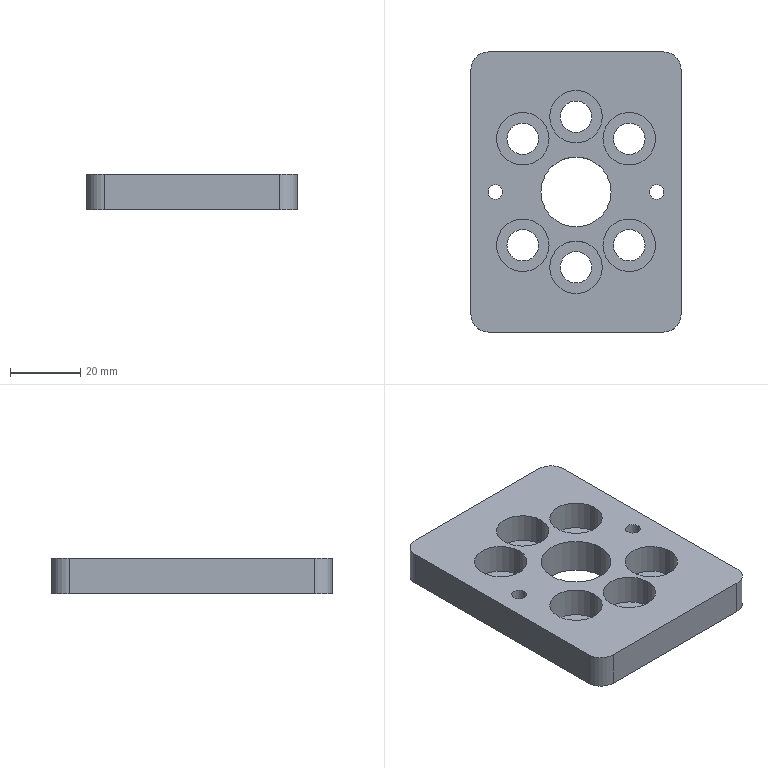Part | SolidWorks | features HoleWzd 2, CirPattern 1, Extrusion 1, Fillet 1 | 1 solid | 46 faces | box 60 x 80 x 10 mm | volume 34714 mm3 | cylinder 34 | plane 12 | commonest cylinder face diameters 9 x12 15 x12 4.2 x4 10 x4 20 x2
STEP:
#1=CARTESIAN_POINT('',(7.703,15.203,1.4));
#2=VERTEX_POINT('',#1);
#3=CARTESIAN_POINT('',(22.703,15.203,1.4));
#4=VERTEX_POINT('',#3);
#5=CARTESIAN_POINT('',(15.203,15.203,1.4));
#6=DIRECTION('',(0.,0.,1.));
#7=DIRECTION('',(1.,0.,0.));
#8=AXIS2_PLACEMENT_3D('',#5,#6,#7);
#9=CIRCLE('',#8,7.5);
#10=EDGE_CURVE('',#2,#4,#9,.T.);
#11=ORIENTED_EDGE('',*,*,#10,.F.);
#12=CARTESIAN_POINT('',(7.703,15.203,10.));
#13=VERTEX_POINT('',#12);
#14=CARTESIAN_POINT('',(7.703,15.203,10.));
#15=DIRECTION('',(0.,0.,1.));
#16=VECTOR('',#15,1000.);
#17=LINE('',#14,#16);
#18=EDGE_CURVE('',#2,#13,#17,.T.);
#19=ORIENTED_EDGE('',*,*,#18,.T.);
#20=CARTESIAN_POINT('',(22.703,15.203,10.));
#21=VERTEX_POINT('',#20);
#22=CARTESIAN_POINT('',(15.203,15.203,10.));
#23=DIRECTION('',(0.,0.,1.));
#24=DIRECTION('',(1.,0.,0.));
#25=AXIS2_PLACEMENT_3D('',#22,#23,#24);
#26=CIRCLE('',#25,7.5);
#27=EDGE_CURVE('',#13,#21,#26,.T.);
#28=ORIENTED_EDGE('',*,*,#27,.T.);
#29=CARTESIAN_POINT('',(22.703,15.203,10.));
#30=DIRECTION('',(0.,0.,1.));
#31=VECTOR('',#30,1000.);
#32=LINE('',#29,#31);
#33=EDGE_CURVE('',#4,#21,#32,.T.);
#34=ORIENTED_EDGE('',*,*,#33,.F.);
#35=EDGE_LOOP('',(#11,#19,#28,#34));
#36=FACE_OUTER_BOUND('',#35,.T.);
#37=CARTESIAN_POINT('',(15.203,15.203,10.));
#38=DIRECTION('',(0.,0.,1.));
#39=DIRECTION('',(1.,0.,0.));
#40=AXIS2_PLACEMENT_3D('',#37,#38,#39);
#41=CYLINDRICAL_SURFACE('',#40,7.5);
#42=ADVANCED_FACE('',(#36),#41,.F.);
#43=CARTESIAN_POINT('',(10.703,15.203,0.));
#44=VERTEX_POINT('',#43);
#45=CARTESIAN_POINT('',(19.703,15.203,0.));
#46=VERTEX_POINT('',#45);
#47=CARTESIAN_POINT('',(15.203,15.203,0.));
#48=DIRECTION('',(0.,0.,1.));
#49=DIRECTION('',(1.,0.,0.));
#50=AXIS2_PLACEMENT_3D('',#47,#48,#49);
#51=CIRCLE('',#50,4.5);
#52=EDGE_CURVE('',#44,#46,#51,.T.);
#53=ORIENTED_EDGE('',*,*,#52,.F.);
#54=CARTESIAN_POINT('',(10.703,15.203,1.4));
#55=VERTEX_POINT('',#54);
#56=CARTESIAN_POINT('',(10.703,15.203,10.));
#57=DIRECTION('',(0.,0.,1.));
#58=VECTOR('',#57,1000.);
#59=LINE('',#56,#58);
#60=EDGE_CURVE('',#44,#55,#59,.T.);
#61=ORIENTED_EDGE('',*,*,#60,.T.);
#62=CARTESIAN_POINT('',(19.703,15.203,1.4));
#63=VERTEX_POINT('',#62);
#64=CARTESIAN_POINT('',(15.203,15.203,1.4));
#65=DIRECTION('',(0.,0.,1.));
#66=DIRECTION('',(1.,0.,0.));
#67=AXIS2_PLACEMENT_3D('',#64,#65,#66);
#68=CIRCLE('',#67,4.5);
#69=EDGE_CURVE('',#55,#63,#68,.T.);
#70=ORIENTED_EDGE('',*,*,#69,.T.);
#71=CARTESIAN_POINT('',(19.703,15.203,10.));
#72=DIRECTION('',(0.,0.,1.));
#73=VECTOR('',#72,1000.);
#74=LINE('',#71,#73);
#75=EDGE_CURVE('',#46,#63,#74,.T.);
#76=ORIENTED_EDGE('',*,*,#75,.F.);
#77=EDGE_LOOP('',(#53,#61,#70,#76));
#78=FACE_OUTER_BOUND('',#77,.T.);
#79=CARTESIAN_POINT('',(15.203,15.203,10.));
#80=DIRECTION('',(0.,0.,1.));
#81=DIRECTION('',(1.,0.,0.));
#82=AXIS2_PLACEMENT_3D('',#79,#80,#81);
#83=CYLINDRICAL_SURFACE('',#82,4.5);
#84=ADVANCED_FACE('',(#78),#83,.F.);
#85=CARTESIAN_POINT('',(7.703,-15.203,1.4));
#86=VERTEX_POINT('',#85);
#87=CARTESIAN_POINT('',(22.703,-15.203,1.4));
#88=VERTEX_POINT('',#87);
#89=CARTESIAN_POINT('',(15.203,-15.203,1.4));
#90=DIRECTION('',(0.,0.,1.));
#91=DIRECTION('',(1.,0.,0.));
#92=AXIS2_PLACEMENT_3D('',#89,#90,#91);
#93=CIRCLE('',#92,7.5);
#94=EDGE_CURVE('',#86,#88,#93,.T.);
#95=ORIENTED_EDGE('',*,*,#94,.F.);
#96=CARTESIAN_POINT('',(7.703,-15.203,10.));
#97=VERTEX_POINT('',#96);
#98=CARTESIAN_POINT('',(7.703,-15.203,10.));
#99=DIRECTION('',(0.,0.,1.));
#100=VECTOR('',#99,1000.);
#101=LINE('',#98,#100);
#102=EDGE_CURVE('',#86,#97,#101,.T.);
#103=ORIENTED_EDGE('',*,*,#102,.T.);
#104=CARTESIAN_POINT('',(22.703,-15.203,10.));
#105=VERTEX_POINT('',#104);
#106=CARTESIAN_POINT('',(15.203,-15.203,10.));
#107=DIRECTION('',(0.,0.,1.));
#108=DIRECTION('',(1.,0.,0.));
#109=AXIS2_PLACEMENT_3D('',#106,#107,#108);
#110=CIRCLE('',#109,7.5);
#111=EDGE_CURVE('',#97,#105,#110,.T.);
#112=ORIENTED_EDGE('',*,*,#111,.T.);
#113=CARTESIAN_POINT('',(22.703,-15.203,10.));
#114=DIRECTION('',(0.,0.,1.));
#115=VECTOR('',#114,1000.);
#116=LINE('',#113,#115);
#117=EDGE_CURVE('',#88,#105,#116,.T.);
#118=ORIENTED_EDGE('',*,*,#117,.F.);
#119=EDGE_LOOP('',(#95,#103,#112,#118));
#120=FACE_OUTER_BOUND('',#119,.T.);
#121=CARTESIAN_POINT('',(15.203,-15.203,10.));
#122=DIRECTION('',(0.,0.,1.));
#123=DIRECTION('',(1.,0.,0.));
#124=AXIS2_PLACEMENT_3D('',#121,#122,#123);
#125=CYLINDRICAL_SURFACE('',#124,7.5);
#126=ADVANCED_FACE('',(#120),#125,.F.);
#127=CARTESIAN_POINT('',(10.703,-15.203,0.));
#128=VERTEX_POINT('',#127);
#129=CARTESIAN_POINT('',(19.703,-15.203,0.));
#130=VERTEX_POINT('',#129);
#131=CARTESIAN_POINT('',(15.203,-15.203,0.));
#132=DIRECTION('',(0.,0.,1.));
#133=DIRECTION('',(1.,0.,0.));
#134=AXIS2_PLACEMENT_3D('',#131,#132,#133);
#135=CIRCLE('',#134,4.5);
#136=EDGE_CURVE('',#128,#130,#135,.T.);
#137=ORIENTED_EDGE('',*,*,#136,.F.);
#138=CARTESIAN_POINT('',(10.703,-15.203,1.4));
#139=VERTEX_POINT('',#138);
#140=CARTESIAN_POINT('',(10.703,-15.203,10.));
#141=DIRECTION('',(0.,0.,1.));
#142=VECTOR('',#141,1000.);
#143=LINE('',#140,#142);
#144=EDGE_CURVE('',#128,#139,#143,.T.);
#145=ORIENTED_EDGE('',*,*,#144,.T.);
#146=CARTESIAN_POINT('',(19.703,-15.203,1.4));
#147=VERTEX_POINT('',#146);
#148=CARTESIAN_POINT('',(15.203,-15.203,1.4));
#149=DIRECTION('',(0.,0.,1.));
#150=DIRECTION('',(1.,0.,0.));
#151=AXIS2_PLACEMENT_3D('',#148,#149,#150);
#152=CIRCLE('',#151,4.5);
#153=EDGE_CURVE('',#139,#147,#152,.T.);
#154=ORIENTED_EDGE('',*,*,#153,.T.);
#155=CARTESIAN_POINT('',(19.703,-15.203,10.));
#156=DIRECTION('',(0.,0.,1.));
#157=VECTOR('',#156,1000.);
#158=LINE('',#155,#157);
#159=EDGE_CURVE('',#130,#147,#158,.T.);
#160=ORIENTED_EDGE('',*,*,#159,.F.);
#161=EDGE_LOOP('',(#137,#145,#154,#160));
#162=FACE_OUTER_BOUND('',#161,.T.);
#163=CARTESIAN_POINT('',(15.203,-15.203,10.));
#164=DIRECTION('',(0.,0.,1.));
#165=DIRECTION('',(1.,0.,0.));
#166=AXIS2_PLACEMENT_3D('',#163,#164,#165);
#167=CYLINDRICAL_SURFACE('',#166,4.5);
#168=ADVANCED_FACE('',(#162),#167,.F.);
#169=CARTESIAN_POINT('',(-7.5,-21.5,1.4));
#170=VERTEX_POINT('',#169);
#171=CARTESIAN_POINT('',(7.5,-21.5,1.4));
#172=VERTEX_POINT('',#171);
#173=CARTESIAN_POINT('',(0.,-21.5,1.4));
#174=DIRECTION('',(0.,0.,1.));
#175=DIRECTION('',(1.,0.,0.));
#176=AXIS2_PLACEMENT_3D('',#173,#174,#175);
#177=CIRCLE('',#176,7.5);
#178=EDGE_CURVE('',#170,#172,#177,.T.);
#179=ORIENTED_EDGE('',*,*,#178,.F.);
#180=CARTESIAN_POINT('',(-7.5,-21.5,10.));
#181=VERTEX_POINT('',#180);
#182=CARTESIAN_POINT('',(-7.5,-21.5,10.));
#183=DIRECTION('',(0.,0.,1.));
#184=VECTOR('',#183,1000.);
#185=LINE('',#182,#184);
#186=EDGE_CURVE('',#170,#181,#185,.T.);
#187=ORIENTED_EDGE('',*,*,#186,.T.);
#188=CARTESIAN_POINT('',(7.5,-21.5,10.));
#189=VERTEX_POINT('',#188);
#190=CARTESIAN_POINT('',(0.,-21.5,10.));
#191=DIRECTION('',(0.,0.,1.));
#192=DIRECTION('',(1.,0.,0.));
#193=AXIS2_PLACEMENT_3D('',#190,#191,#192);
#194=CIRCLE('',#193,7.5);
#195=EDGE_CURVE('',#181,#189,#194,.T.);
#196=ORIENTED_EDGE('',*,*,#195,.T.);
#197=CARTESIAN_POINT('',(7.5,-21.5,10.));
#198=DIRECTION('',(0.,0.,1.));
#199=VECTOR('',#198,1000.);
#200=LINE('',#197,#199);
#201=EDGE_CURVE('',#172,#189,#200,.T.);
#202=ORIENTED_EDGE('',*,*,#201,.F.);
#203=EDGE_LOOP('',(#179,#187,#196,#202));
#204=FACE_OUTER_BOUND('',#203,.T.);
#205=CARTESIAN_POINT('',(0.,-21.5,10.));
#206=DIRECTION('',(0.,0.,1.));
#207=DIRECTION('',(1.,0.,0.));
#208=AXIS2_PLACEMENT_3D('',#205,#206,#207);
#209=CYLINDRICAL_SURFACE('',#208,7.5);
#210=ADVANCED_FACE('',(#204),#209,.F.);
#211=CARTESIAN_POINT('',(-4.5,-21.5,0.));
#212=VERTEX_POINT('',#211);
#213=CARTESIAN_POINT('',(4.5,-21.5,0.));
#214=VERTEX_POINT('',#213);
#215=CARTESIAN_POINT('',(0.,-21.5,0.));
#216=DIRECTION('',(0.,0.,1.));
#217=DIRECTION('',(1.,0.,0.));
#218=AXIS2_PLACEMENT_3D('',#215,#216,#217);
#219=CIRCLE('',#218,4.5);
#220=EDGE_CURVE('',#212,#214,#219,.T.);
#221=ORIENTED_EDGE('',*,*,#220,.F.);
#222=CARTESIAN_POINT('',(-4.5,-21.5,1.4));
#223=VERTEX_POINT('',#222);
#224=CARTESIAN_POINT('',(-4.5,-21.5,10.));
#225=DIRECTION('',(0.,0.,1.));
#226=VECTOR('',#225,1000.);
#227=LINE('',#224,#226);
#228=EDGE_CURVE('',#212,#223,#227,.T.);
#229=ORIENTED_EDGE('',*,*,#228,.T.);
#230=CARTESIAN_POINT('',(4.5,-21.5,1.4));
#231=VERTEX_POINT('',#230);
#232=CARTESIAN_POINT('',(0.,-21.5,1.4));
#233=DIRECTION('',(0.,0.,1.));
#234=DIRECTION('',(1.,0.,0.));
#235=AXIS2_PLACEMENT_3D('',#232,#233,#234);
#236=CIRCLE('',#235,4.5);
#237=EDGE_CURVE('',#223,#231,#236,.T.);
#238=ORIENTED_EDGE('',*,*,#237,.T.);
#239=CARTESIAN_POINT('',(4.5,-21.5,10.));
#240=DIRECTION('',(0.,0.,1.));
#241=VECTOR('',#240,1000.);
#242=LINE('',#239,#241);
#243=EDGE_CURVE('',#214,#231,#242,.T.);
#244=ORIENTED_EDGE('',*,*,#243,.F.);
#245=EDGE_LOOP('',(#221,#229,#238,#244));
#246=FACE_OUTER_BOUND('',#245,.T.);
#247=CARTESIAN_POINT('',(0.,-21.5,10.));
#248=DIRECTION('',(0.,0.,1.));
#249=DIRECTION('',(1.,0.,0.));
#250=AXIS2_PLACEMENT_3D('',#247,#248,#249);
#251=CYLINDRICAL_SURFACE('',#250,4.5);
#252=ADVANCED_FACE('',(#246),#251,.F.);
#253=CARTESIAN_POINT('',(-22.703,-15.203,1.4));
#254=VERTEX_POINT('',#253);
#255=CARTESIAN_POINT('',(-7.703,-15.203,1.4));
#256=VERTEX_POINT('',#255);
#257=CARTESIAN_POINT('',(-15.203,-15.203,1.4));
#258=DIRECTION('',(0.,0.,1.));
#259=DIRECTION('',(1.,0.,0.));
#260=AXIS2_PLACEMENT_3D('',#257,#258,#259);
#261=CIRCLE('',#260,7.5);
#262=EDGE_CURVE('',#254,#256,#261,.T.);
#263=ORIENTED_EDGE('',*,*,#262,.F.);
#264=CARTESIAN_POINT('',(-22.703,-15.203,10.));
#265=VERTEX_POINT('',#264);
#266=CARTESIAN_POINT('',(-22.703,-15.203,10.));
#267=DIRECTION('',(0.,0.,1.));
#268=VECTOR('',#267,1000.);
#269=LINE('',#266,#268);
#270=EDGE_CURVE('',#254,#265,#269,.T.);
#271=ORIENTED_EDGE('',*,*,#270,.T.);
#272=CARTESIAN_POINT('',(-7.703,-15.203,10.));
#273=VERTEX_POINT('',#272);
#274=CARTESIAN_POINT('',(-15.203,-15.203,10.));
#275=DIRECTION('',(0.,0.,1.));
#276=DIRECTION('',(1.,0.,0.));
#277=AXIS2_PLACEMENT_3D('',#274,#275,#276);
#278=CIRCLE('',#277,7.5);
#279=EDGE_CURVE('',#265,#273,#278,.T.);
#280=ORIENTED_EDGE('',*,*,#279,.T.);
#281=CARTESIAN_POINT('',(-7.703,-15.203,10.));
#282=DIRECTION('',(0.,0.,1.));
#283=VECTOR('',#282,1000.);
#284=LINE('',#281,#283);
#285=EDGE_CURVE('',#256,#273,#284,.T.);
#286=ORIENTED_EDGE('',*,*,#285,.F.);
#287=EDGE_LOOP('',(#263,#271,#280,#286));
#288=FACE_OUTER_BOUND('',#287,.T.);
#289=CARTESIAN_POINT('',(-15.203,-15.203,10.));
#290=DIRECTION('',(0.,0.,1.));
#291=DIRECTION('',(1.,0.,0.));
#292=AXIS2_PLACEMENT_3D('',#289,#290,#291);
#293=CYLINDRICAL_SURFACE('',#292,7.5);
#294=ADVANCED_FACE('',(#288),#293,.F.);
#295=CARTESIAN_POINT('',(-19.703,-15.203,0.));
#296=VERTEX_POINT('',#295);
#297=CARTESIAN_POINT('',(-10.703,-15.203,0.));
#298=VERTEX_POINT('',#297);
#299=CARTESIAN_POINT('',(-15.203,-15.203,0.));
#300=DIRECTION('',(0.,0.,1.));
#301=DIRECTION('',(1.,0.,0.));
#302=AXIS2_PLACEMENT_3D('',#299,#300,#301);
#303=CIRCLE('',#302,4.5);
#304=EDGE_CURVE('',#296,#298,#303,.T.);
#305=ORIENTED_EDGE('',*,*,#304,.F.);
#306=CARTESIAN_POINT('',(-19.703,-15.203,1.4));
#307=VERTEX_POINT('',#306);
#308=CARTESIAN_POINT('',(-19.703,-15.203,10.));
#309=DIRECTION('',(0.,0.,1.));
#310=VECTOR('',#309,1000.);
#311=LINE('',#308,#310);
#312=EDGE_CURVE('',#296,#307,#311,.T.);
#313=ORIENTED_EDGE('',*,*,#312,.T.);
#314=CARTESIAN_POINT('',(-10.703,-15.203,1.4));
#315=VERTEX_POINT('',#314);
#316=CARTESIAN_POINT('',(-15.203,-15.203,1.4));
#317=DIRECTION('',(0.,0.,1.));
#318=DIRECTION('',(1.,0.,0.));
#319=AXIS2_PLACEMENT_3D('',#316,#317,#318);
#320=CIRCLE('',#319,4.5);
#321=EDGE_CURVE('',#307,#315,#320,.T.);
#322=ORIENTED_EDGE('',*,*,#321,.T.);
#323=CARTESIAN_POINT('',(-10.703,-15.203,10.));
#324=DIRECTION('',(0.,0.,1.));
#325=VECTOR('',#324,1000.);
#326=LINE('',#323,#325);
#327=EDGE_CURVE('',#298,#315,#326,.T.);
#328=ORIENTED_EDGE('',*,*,#327,.F.);
#329=EDGE_LOOP('',(#305,#313,#322,#328));
#330=FACE_OUTER_BOUND('',#329,.T.);
#331=CARTESIAN_POINT('',(-15.203,-15.203,10.));
#332=DIRECTION('',(0.,0.,1.));
#333=DIRECTION('',(1.,0.,0.));
#334=AXIS2_PLACEMENT_3D('',#331,#332,#333);
#335=CYLINDRICAL_SURFACE('',#334,4.5);
#336=ADVANCED_FACE('',(#330),#335,.F.);
#337=CARTESIAN_POINT('',(-22.703,15.203,1.4));
#338=VERTEX_POINT('',#337);
#339=CARTESIAN_POINT('',(-7.703,15.203,1.4));
#340=VERTEX_POINT('',#339);
#341=CARTESIAN_POINT('',(-15.203,15.203,1.4));
#342=DIRECTION('',(0.,0.,1.));
#343=DIRECTION('',(1.,0.,0.));
#344=AXIS2_PLACEMENT_3D('',#341,#342,#343);
#345=CIRCLE('',#344,7.5);
#346=EDGE_CURVE('',#338,#340,#345,.T.);
#347=ORIENTED_EDGE('',*,*,#346,.F.);
#348=CARTESIAN_POINT('',(-22.703,15.203,10.));
#349=VERTEX_POINT('',#348);
#350=CARTESIAN_POINT('',(-22.703,15.203,10.));
#351=DIRECTION('',(0.,0.,1.));
#352=VECTOR('',#351,1000.);
#353=LINE('',#350,#352);
#354=EDGE_CURVE('',#338,#349,#353,.T.);
#355=ORIENTED_EDGE('',*,*,#354,.T.);
#356=CARTESIAN_POINT('',(-7.703,15.203,10.));
#357=VERTEX_POINT('',#356);
#358=CARTESIAN_POINT('',(-15.203,15.203,10.));
#359=DIRECTION('',(0.,0.,1.));
#360=DIRECTION('',(1.,0.,0.));
#361=AXIS2_PLACEMENT_3D('',#358,#359,#360);
#362=CIRCLE('',#361,7.5);
#363=EDGE_CURVE('',#349,#357,#362,.T.);
#364=ORIENTED_EDGE('',*,*,#363,.T.);
#365=CARTESIAN_POINT('',(-7.703,15.203,10.));
#366=DIRECTION('',(0.,0.,1.));
#367=VECTOR('',#366,1000.);
#368=LINE('',#365,#367);
#369=EDGE_CURVE('',#340,#357,#368,.T.);
#370=ORIENTED_EDGE('',*,*,#369,.F.);
#371=EDGE_LOOP('',(#347,#355,#364,#370));
#372=FACE_OUTER_BOUND('',#371,.T.);
#373=CARTESIAN_POINT('',(-15.203,15.203,10.));
#374=DIRECTION('',(0.,0.,1.));
#375=DIRECTION('',(1.,0.,0.));
#376=AXIS2_PLACEMENT_3D('',#373,#374,#375);
#377=CYLINDRICAL_SURFACE('',#376,7.5);
#378=ADVANCED_FACE('',(#372),#377,.F.);
#379=CARTESIAN_POINT('',(-19.703,15.203,0.));
#380=VERTEX_POINT('',#379);
#381=CARTESIAN_POINT('',(-10.703,15.203,0.));
#382=VERTEX_POINT('',#381);
#383=CARTESIAN_POINT('',(-15.203,15.203,0.));
#384=DIRECTION('',(0.,0.,1.));
#385=DIRECTION('',(1.,0.,0.));
#386=AXIS2_PLACEMENT_3D('',#383,#384,#385);
#387=CIRCLE('',#386,4.5);
#388=EDGE_CURVE('',#380,#382,#387,.T.);
#389=ORIENTED_EDGE('',*,*,#388,.F.);
#390=CARTESIAN_POINT('',(-19.703,15.203,1.4));
#391=VERTEX_POINT('',#390);
#392=CARTESIAN_POINT('',(-19.703,15.203,10.));
#393=DIRECTION('',(0.,0.,1.));
#394=VECTOR('',#393,1000.);
#395=LINE('',#392,#394);
#396=EDGE_CURVE('',#380,#391,#395,.T.);
#397=ORIENTED_EDGE('',*,*,#396,.T.);
#398=CARTESIAN_POINT('',(-10.703,15.203,1.4));
#399=VERTEX_POINT('',#398);
#400=CARTESIAN_POINT('',(-15.203,15.203,1.4));
#401=DIRECTION('',(0.,0.,1.));
#402=DIRECTION('',(1.,0.,0.));
#403=AXIS2_PLACEMENT_3D('',#400,#401,#402);
#404=CIRCLE('',#403,4.5);
#405=EDGE_CURVE('',#391,#399,#404,.T.);
#406=ORIENTED_EDGE('',*,*,#405,.T.);
#407=CARTESIAN_POINT('',(-10.703,15.203,10.));
#408=DIRECTION('',(0.,0.,1.));
#409=VECTOR('',#408,1000.);
#410=LINE('',#407,#409);
#411=EDGE_CURVE('',#382,#399,#410,.T.);
#412=ORIENTED_EDGE('',*,*,#411,.F.);
#413=EDGE_LOOP('',(#389,#397,#406,#412));
#414=FACE_OUTER_BOUND('',#413,.T.);
#415=CARTESIAN_POINT('',(-15.203,15.203,10.));
#416=DIRECTION('',(0.,0.,1.));
#417=DIRECTION('',(1.,0.,0.));
#418=AXIS2_PLACEMENT_3D('',#415,#416,#417);
#419=CYLINDRICAL_SURFACE('',#418,4.5);
#420=ADVANCED_FACE('',(#414),#419,.F.);
#421=CARTESIAN_POINT('',(-7.5,21.5,1.4));
#422=VERTEX_POINT('',#421);
#423=CARTESIAN_POINT('',(7.5,21.5,1.4));
#424=VERTEX_POINT('',#423);
#425=CARTESIAN_POINT('',(0.,21.5,1.4));
#426=DIRECTION('',(0.,0.,1.));
#427=DIRECTION('',(1.,0.,0.));
#428=AXIS2_PLACEMENT_3D('',#425,#426,#427);
#429=CIRCLE('',#428,7.5);
#430=EDGE_CURVE('',#422,#424,#429,.T.);
#431=ORIENTED_EDGE('',*,*,#430,.F.);
#432=CARTESIAN_POINT('',(-7.5,21.5,10.));
#433=VERTEX_POINT('',#432);
#434=CARTESIAN_POINT('',(-7.5,21.5,10.));
#435=DIRECTION('',(0.,0.,1.));
#436=VECTOR('',#435,1000.);
#437=LINE('',#434,#436);
#438=EDGE_CURVE('',#422,#433,#437,.T.);
#439=ORIENTED_EDGE('',*,*,#438,.T.);
#440=CARTESIAN_POINT('',(7.5,21.5,10.));
#441=VERTEX_POINT('',#440);
#442=CARTESIAN_POINT('',(0.,21.5,10.));
#443=DIRECTION('',(0.,0.,1.));
#444=DIRECTION('',(1.,0.,0.));
#445=AXIS2_PLACEMENT_3D('',#442,#443,#444);
#446=CIRCLE('',#445,7.5);
#447=EDGE_CURVE('',#433,#441,#446,.T.);
#448=ORIENTED_EDGE('',*,*,#447,.T.);
#449=CARTESIAN_POINT('',(7.5,21.5,10.));
#450=DIRECTION('',(0.,0.,1.));
#451=VECTOR('',#450,1000.);
#452=LINE('',#449,#451);
#453=EDGE_CURVE('',#424,#441,#452,.T.);
#454=ORIENTED_EDGE('',*,*,#453,.F.);
#455=EDGE_LOOP('',(#431,#439,#448,#454));
#456=FACE_OUTER_BOUND('',#455,.T.);
#457=CARTESIAN_POINT('',(0.,21.5,10.));
#458=DIRECTION('',(0.,0.,1.));
#459=DIRECTION('',(1.,0.,0.));
#460=AXIS2_PLACEMENT_3D('',#457,#458,#459);
#461=CYLINDRICAL_SURFACE('',#460,7.5);
#462=ADVANCED_FACE('',(#456),#461,.F.);
#463=CARTESIAN_POINT('',(-4.5,21.5,0.));
#464=VERTEX_POINT('',#463);
#465=CARTESIAN_POINT('',(4.5,21.5,0.));
#466=VERTEX_POINT('',#465);
#467=CARTESIAN_POINT('',(0.,21.5,0.));
#468=DIRECTION('',(0.,0.,1.));
#469=DIRECTION('',(1.,0.,0.));
#470=AXIS2_PLACEMENT_3D('',#467,#468,#469);
#471=CIRCLE('',#470,4.5);
#472=EDGE_CURVE('',#464,#466,#471,.T.);
#473=ORIENTED_EDGE('',*,*,#472,.F.);
#474=CARTESIAN_POINT('',(-4.5,21.5,1.4));
#475=VERTEX_POINT('',#474);
#476=CARTESIAN_POINT('',(-4.5,21.5,10.));
#477=DIRECTION('',(0.,0.,1.));
#478=VECTOR('',#477,1000.);
#479=LINE('',#476,#478);
#480=EDGE_CURVE('',#464,#475,#479,.T.);
#481=ORIENTED_EDGE('',*,*,#480,.T.);
#482=CARTESIAN_POINT('',(4.5,21.5,1.4));
#483=VERTEX_POINT('',#482);
#484=CARTESIAN_POINT('',(0.,21.5,1.4));
#485=DIRECTION('',(0.,0.,1.));
#486=DIRECTION('',(1.,0.,0.));
#487=AXIS2_PLACEMENT_3D('',#484,#485,#486);
#488=CIRCLE('',#487,4.5);
#489=EDGE_CURVE('',#475,#483,#488,.T.);
#490=ORIENTED_EDGE('',*,*,#489,.T.);
#491=CARTESIAN_POINT('',(4.5,21.5,10.));
#492=DIRECTION('',(0.,0.,1.));
#493=VECTOR('',#492,1000.);
#494=LINE('',#491,#493);
#495=EDGE_CURVE('',#466,#483,#494,.T.);
#496=ORIENTED_EDGE('',*,*,#495,.F.);
#497=EDGE_LOOP('',(#473,#481,#490,#496));
#498=FACE_OUTER_BOUND('',#497,.T.);
#499=CARTESIAN_POINT('',(0.,21.5,10.));
#500=DIRECTION('',(0.,0.,1.));
#501=DIRECTION('',(1.,0.,0.));
#502=AXIS2_PLACEMENT_3D('',#499,#500,#501);
#503=CYLINDRICAL_SURFACE('',#502,4.5);
#504=ADVANCED_FACE('',(#498),#503,.F.);
#505=CARTESIAN_POINT('',(-25.1,0.,0.));
#506=VERTEX_POINT('',#505);
#507=CARTESIAN_POINT('',(-20.9,0.,0.));
#508=VERTEX_POINT('',#507);
#509=CARTESIAN_POINT('',(-23.,0.,0.));
#510=DIRECTION('',(0.,0.,1.));
#511=DIRECTION('',(1.,0.,0.));
#512=AXIS2_PLACEMENT_3D('',#509,#510,#511);
#513=CIRCLE('',#512,2.1);
#514=EDGE_CURVE('',#506,#508,#513,.T.);
#515=ORIENTED_EDGE('',*,*,#514,.F.);
#516=CARTESIAN_POINT('',(-25.1,0.,10.));
#517=VERTEX_POINT('',#516);
#518=CARTESIAN_POINT('',(-25.1,0.,10.));
#519=DIRECTION('',(0.,0.,1.));
#520=VECTOR('',#519,1000.);
#521=LINE('',#518,#520);
#522=EDGE_CURVE('',#506,#517,#521,.T.);
#523=ORIENTED_EDGE('',*,*,#522,.T.);
#524=CARTESIAN_POINT('',(-20.9,0.,10.));
#525=VERTEX_POINT('',#524);
#526=CARTESIAN_POINT('',(-23.,0.,10.));
#527=DIRECTION('',(0.,0.,1.));
#528=DIRECTION('',(1.,0.,0.));
#529=AXIS2_PLACEMENT_3D('',#526,#527,#528);
#530=CIRCLE('',#529,2.1);
#531=EDGE_CURVE('',#517,#525,#530,.T.);
#532=ORIENTED_EDGE('',*,*,#531,.T.);
#533=CARTESIAN_POINT('',(-20.9,0.,10.));
#534=DIRECTION('',(0.,0.,1.));
#535=VECTOR('',#534,1000.);
#536=LINE('',#533,#535);
#537=EDGE_CURVE('',#508,#525,#536,.T.);
#538=ORIENTED_EDGE('',*,*,#537,.F.);
#539=EDGE_LOOP('',(#515,#523,#532,#538));
#540=FACE_OUTER_BOUND('',#539,.T.);
#541=CARTESIAN_POINT('',(-23.,0.,10.));
#542=DIRECTION('',(0.,0.,1.));
#543=DIRECTION('',(1.,0.,0.));
#544=AXIS2_PLACEMENT_3D('',#541,#542,#543);
#545=CYLINDRICAL_SURFACE('',#544,2.1);
#546=ADVANCED_FACE('',(#540),#545,.F.);
#547=CARTESIAN_POINT('',(20.9,0.,0.));
#548=VERTEX_POINT('',#547);
#549=CARTESIAN_POINT('',(25.1,0.,0.));
#550=VERTEX_POINT('',#549);
#551=CARTESIAN_POINT('',(23.,0.,0.));
#552=DIRECTION('',(0.,0.,1.));
#553=DIRECTION('',(1.,0.,0.));
#554=AXIS2_PLACEMENT_3D('',#551,#552,#553);
#555=CIRCLE('',#554,2.1);
#556=EDGE_CURVE('',#548,#550,#555,.T.);
#557=ORIENTED_EDGE('',*,*,#556,.F.);
#558=CARTESIAN_POINT('',(20.9,0.,10.));
#559=VERTEX_POINT('',#558);
#560=CARTESIAN_POINT('',(20.9,0.,10.));
#561=DIRECTION('',(0.,0.,1.));
#562=VECTOR('',#561,1000.);
#563=LINE('',#560,#562);
#564=EDGE_CURVE('',#548,#559,#563,.T.);
#565=ORIENTED_EDGE('',*,*,#564,.T.);
#566=CARTESIAN_POINT('',(25.1,0.,10.));
#567=VERTEX_POINT('',#566);
#568=CARTESIAN_POINT('',(23.,0.,10.));
#569=DIRECTION('',(0.,0.,1.));
#570=DIRECTION('',(1.,0.,0.));
#571=AXIS2_PLACEMENT_3D('',#568,#569,#570);
#572=CIRCLE('',#571,2.1);
#573=EDGE_CURVE('',#559,#567,#572,.T.);
#574=ORIENTED_EDGE('',*,*,#573,.T.);
#575=CARTESIAN_POINT('',(25.1,0.,10.));
#576=DIRECTION('',(0.,0.,1.));
#577=VECTOR('',#576,1000.);
#578=LINE('',#575,#577);
#579=EDGE_CURVE('',#550,#567,#578,.T.);
#580=ORIENTED_EDGE('',*,*,#579,.F.);
#581=EDGE_LOOP('',(#557,#565,#574,#580));
#582=FACE_OUTER_BOUND('',#581,.T.);
#583=CARTESIAN_POINT('',(23.,0.,10.));
#584=DIRECTION('',(0.,0.,1.));
#585=DIRECTION('',(1.,0.,0.));
#586=AXIS2_PLACEMENT_3D('',#583,#584,#585);
#587=CYLINDRICAL_SURFACE('',#586,2.1);
#588=ADVANCED_FACE('',(#582),#587,.F.);
#589=CARTESIAN_POINT('',(-10.,0.,10.));
#590=VERTEX_POINT('',#589);
#591=CARTESIAN_POINT('',(10.,0.,10.));
#592=VERTEX_POINT('',#591);
#593=CARTESIAN_POINT('',(0.,0.,10.));
#594=DIRECTION('',(0.,0.,1.));
#595=DIRECTION('',(1.,0.,0.));
#596=AXIS2_PLACEMENT_3D('',#593,#594,#595);
#597=CIRCLE('',#596,10.);
#598=EDGE_CURVE('',#590,#592,#597,.T.);
#599=ORIENTED_EDGE('',*,*,#598,.T.);
#600=CARTESIAN_POINT('',(10.,0.,0.));
#601=VERTEX_POINT('',#600);
#602=CARTESIAN_POINT('',(10.,0.,10.));
#603=DIRECTION('',(0.,0.,-1.));
#604=VECTOR('',#603,1000.);
#605=LINE('',#602,#604);
#606=EDGE_CURVE('',#592,#601,#605,.T.);
#607=ORIENTED_EDGE('',*,*,#606,.T.);
#608=CARTESIAN_POINT('',(-10.,0.,0.));
#609=VERTEX_POINT('',#608);
#610=CARTESIAN_POINT('',(0.,0.,0.));
#611=DIRECTION('',(0.,0.,1.));
#612=DIRECTION('',(1.,0.,0.));
#613=AXIS2_PLACEMENT_3D('',#610,#611,#612);
#614=CIRCLE('',#613,10.);
#615=EDGE_CURVE('',#609,#601,#614,.T.);
#616=ORIENTED_EDGE('',*,*,#615,.F.);
#617=CARTESIAN_POINT('',(-10.,0.,10.));
#618=DIRECTION('',(0.,0.,-1.));
#619=VECTOR('',#618,1000.);
#620=LINE('',#617,#619);
#621=EDGE_CURVE('',#590,#609,#620,.T.);
#622=ORIENTED_EDGE('',*,*,#621,.F.);
#623=EDGE_LOOP('',(#599,#607,#616,#622));
#624=FACE_OUTER_BOUND('',#623,.T.);
#625=CARTESIAN_POINT('',(0.,0.,10.));
#626=DIRECTION('',(0.,0.,-1.));
#627=DIRECTION('',(-1.,0.,0.));
#628=AXIS2_PLACEMENT_3D('',#625,#626,#627);
#629=CYLINDRICAL_SURFACE('',#628,10.);
#630=ADVANCED_FACE('',(#624),#629,.F.);
#631=CARTESIAN_POINT('',(15.203,15.203,10.));
#632=DIRECTION('',(0.,0.,1.));
#633=DIRECTION('',(1.,0.,0.));
#634=AXIS2_PLACEMENT_3D('',#631,#632,#633);
#635=CIRCLE('',#634,7.5);
#636=EDGE_CURVE('',#21,#13,#635,.T.);
#637=ORIENTED_EDGE('',*,*,#636,.F.);
#638=ORIENTED_EDGE('',*,*,#27,.F.);
#639=EDGE_LOOP('',(#637,#638));
#640=FACE_BOUND('',#639,.T.);
#641=CARTESIAN_POINT('',(15.203,-15.203,10.));
#642=DIRECTION('',(0.,0.,1.));
#643=DIRECTION('',(1.,0.,0.));
#644=AXIS2_PLACEMENT_3D('',#641,#642,#643);
#645=CIRCLE('',#644,7.5);
#646=EDGE_CURVE('',#105,#97,#645,.T.);
#647=ORIENTED_EDGE('',*,*,#646,.F.);
#648=ORIENTED_EDGE('',*,*,#111,.F.);
#649=EDGE_LOOP('',(#647,#648));
#650=FACE_BOUND('',#649,.T.);
#651=CARTESIAN_POINT('',(0.,-21.5,10.));
#652=DIRECTION('',(0.,0.,1.));
#653=DIRECTION('',(1.,0.,0.));
#654=AXIS2_PLACEMENT_3D('',#651,#652,#653);
#655=CIRCLE('',#654,7.5);
#656=EDGE_CURVE('',#189,#181,#655,.T.);
#657=ORIENTED_EDGE('',*,*,#656,.F.);
#658=ORIENTED_EDGE('',*,*,#195,.F.);
#659=EDGE_LOOP('',(#657,#658));
#660=FACE_BOUND('',#659,.T.);
#661=CARTESIAN_POINT('',(-15.203,-15.203,10.));
#662=DIRECTION('',(0.,0.,1.));
#663=DIRECTION('',(1.,0.,0.));
#664=AXIS2_PLACEMENT_3D('',#661,#662,#663);
#665=CIRCLE('',#664,7.5);
#666=EDGE_CURVE('',#273,#265,#665,.T.);
#667=ORIENTED_EDGE('',*,*,#666,.F.);
#668=ORIENTED_EDGE('',*,*,#279,.F.);
#669=EDGE_LOOP('',(#667,#668));
#670=FACE_BOUND('',#669,.T.);
#671=CARTESIAN_POINT('',(-15.203,15.203,10.));
#672=DIRECTION('',(0.,0.,1.));
#673=DIRECTION('',(1.,0.,0.));
#674=AXIS2_PLACEMENT_3D('',#671,#672,#673);
#675=CIRCLE('',#674,7.5);
#676=EDGE_CURVE('',#357,#349,#675,.T.);
#677=ORIENTED_EDGE('',*,*,#676,.F.);
#678=ORIENTED_EDGE('',*,*,#363,.F.);
#679=EDGE_LOOP('',(#677,#678));
#680=FACE_BOUND('',#679,.T.);
#681=CARTESIAN_POINT('',(0.,21.5,10.));
#682=DIRECTION('',(0.,0.,1.));
#683=DIRECTION('',(1.,0.,0.));
#684=AXIS2_PLACEMENT_3D('',#681,#682,#683);
#685=CIRCLE('',#684,7.5);
#686=EDGE_CURVE('',#441,#433,#685,.T.);
#687=ORIENTED_EDGE('',*,*,#686,.F.);
#688=ORIENTED_EDGE('',*,*,#447,.F.);
#689=EDGE_LOOP('',(#687,#688));
#690=FACE_BOUND('',#689,.T.);
#691=CARTESIAN_POINT('',(-23.,0.,10.));
#692=DIRECTION('',(0.,0.,1.));
#693=DIRECTION('',(1.,0.,0.));
#694=AXIS2_PLACEMENT_3D('',#691,#692,#693);
#695=CIRCLE('',#694,2.1);
#696=EDGE_CURVE('',#525,#517,#695,.T.);
#697=ORIENTED_EDGE('',*,*,#696,.F.);
#698=ORIENTED_EDGE('',*,*,#531,.F.);
#699=EDGE_LOOP('',(#697,#698));
#700=FACE_BOUND('',#699,.T.);
#701=CARTESIAN_POINT('',(23.,0.,10.));
#702=DIRECTION('',(0.,0.,1.));
#703=DIRECTION('',(1.,0.,0.));
#704=AXIS2_PLACEMENT_3D('',#701,#702,#703);
#705=CIRCLE('',#704,2.1);
#706=EDGE_CURVE('',#567,#559,#705,.T.);
#707=ORIENTED_EDGE('',*,*,#706,.F.);
#708=ORIENTED_EDGE('',*,*,#573,.F.);
#709=EDGE_LOOP('',(#707,#708));
#710=FACE_BOUND('',#709,.T.);
#711=CARTESIAN_POINT('',(-25.,-40.,10.));
#712=VERTEX_POINT('',#711);
#713=CARTESIAN_POINT('',(25.,-40.,10.));
#714=VERTEX_POINT('',#713);
#715=CARTESIAN_POINT('',(-30.,-40.,10.));
#716=DIRECTION('',(1.,0.,0.));
#717=VECTOR('',#716,1000.);
#718=LINE('',#715,#717);
#719=EDGE_CURVE('',#712,#714,#718,.T.);
#720=ORIENTED_EDGE('',*,*,#719,.T.);
#721=CARTESIAN_POINT('',(30.,-35.,10.));
#722=VERTEX_POINT('',#721);
#723=CARTESIAN_POINT('',(25.,-35.,10.));
#724=DIRECTION('',(0.,0.,1.));
#725=DIRECTION('',(-1.,0.,0.));
#726=AXIS2_PLACEMENT_3D('',#723,#724,#725);
#727=CIRCLE('',#726,5.);
#728=EDGE_CURVE('',#714,#722,#727,.T.);
#729=ORIENTED_EDGE('',*,*,#728,.T.);
#730=CARTESIAN_POINT('',(30.,35.,10.));
#731=VERTEX_POINT('',#730);
#732=CARTESIAN_POINT('',(30.,-40.,10.));
#733=DIRECTION('',(0.,1.,0.));
#734=VECTOR('',#733,1000.);
#735=LINE('',#732,#734);
#736=EDGE_CURVE('',#722,#731,#735,.T.);
#737=ORIENTED_EDGE('',*,*,#736,.T.);
#738=CARTESIAN_POINT('',(25.,40.,10.));
#739=VERTEX_POINT('',#738);
#740=CARTESIAN_POINT('',(25.,35.,10.));
#741=DIRECTION('',(0.,0.,1.));
#742=DIRECTION('',(-1.,0.,0.));
#743=AXIS2_PLACEMENT_3D('',#740,#741,#742);
#744=CIRCLE('',#743,5.);
#745=EDGE_CURVE('',#731,#739,#744,.T.);
#746=ORIENTED_EDGE('',*,*,#745,.T.);
#747=CARTESIAN_POINT('',(-25.,40.,10.));
#748=VERTEX_POINT('',#747);
#749=CARTESIAN_POINT('',(-30.,40.,10.));
#750=DIRECTION('',(-1.,0.,0.));
#751=VECTOR('',#750,1000.);
#752=LINE('',#749,#751);
#753=EDGE_CURVE('',#739,#748,#752,.T.);
#754=ORIENTED_EDGE('',*,*,#753,.T.);
#755=CARTESIAN_POINT('',(-30.,35.,10.));
#756=VERTEX_POINT('',#755);
#757=CARTESIAN_POINT('',(-25.,35.,10.));
#758=DIRECTION('',(0.,0.,1.));
#759=DIRECTION('',(-1.,0.,0.));
#760=AXIS2_PLACEMENT_3D('',#757,#758,#759);
#761=CIRCLE('',#760,5.);
#762=EDGE_CURVE('',#748,#756,#761,.T.);
#763=ORIENTED_EDGE('',*,*,#762,.T.);
#764=CARTESIAN_POINT('',(-30.,-35.,10.));
#765=VERTEX_POINT('',#764);
#766=CARTESIAN_POINT('',(-30.,-40.,10.));
#767=DIRECTION('',(0.,-1.,0.));
#768=VECTOR('',#767,1000.);
#769=LINE('',#766,#768);
#770=EDGE_CURVE('',#756,#765,#769,.T.);
#771=ORIENTED_EDGE('',*,*,#770,.T.);
#772=CARTESIAN_POINT('',(-25.,-35.,10.));
#773=DIRECTION('',(0.,0.,1.));
#774=DIRECTION('',(-1.,0.,0.));
#775=AXIS2_PLACEMENT_3D('',#772,#773,#774);
#776=CIRCLE('',#775,5.);
#777=EDGE_CURVE('',#765,#712,#776,.T.);
#778=ORIENTED_EDGE('',*,*,#777,.T.);
#779=EDGE_LOOP('',(#720,#729,#737,#746,#754,#763,#771,#778));
#780=FACE_OUTER_BOUND('',#779,.T.);
#781=ORIENTED_EDGE('',*,*,#598,.F.);
#782=CARTESIAN_POINT('',(0.,0.,10.));
#783=DIRECTION('',(0.,0.,1.));
#784=DIRECTION('',(1.,0.,0.));
#785=AXIS2_PLACEMENT_3D('',#782,#783,#784);
#786=CIRCLE('',#785,10.);
#787=EDGE_CURVE('',#592,#590,#786,.T.);
#788=ORIENTED_EDGE('',*,*,#787,.F.);
#789=EDGE_LOOP('',(#781,#788));
#790=FACE_BOUND('',#789,.T.);
#791=CARTESIAN_POINT('',(0.,0.,10.));
#792=DIRECTION('',(0.,0.,-1.));
#793=DIRECTION('',(-1.,0.,0.));
#794=AXIS2_PLACEMENT_3D('',#791,#792,#793);
#795=PLANE('',#794);
#796=ADVANCED_FACE('',(#640,#650,#660,#670,#680,#690,#700,#710,#780,#790),#795,.F.);
#797=CARTESIAN_POINT('',(15.203,15.203,0.));
#798=DIRECTION('',(0.,0.,1.));
#799=DIRECTION('',(1.,0.,0.));
#800=AXIS2_PLACEMENT_3D('',#797,#798,#799);
#801=CIRCLE('',#800,4.5);
#802=EDGE_CURVE('',#46,#44,#801,.T.);
#803=ORIENTED_EDGE('',*,*,#802,.T.);
#804=ORIENTED_EDGE('',*,*,#52,.T.);
#805=EDGE_LOOP('',(#803,#804));
#806=FACE_BOUND('',#805,.T.);
#807=CARTESIAN_POINT('',(15.203,-15.203,0.));
#808=DIRECTION('',(0.,0.,1.));
#809=DIRECTION('',(1.,0.,0.));
#810=AXIS2_PLACEMENT_3D('',#807,#808,#809);
#811=CIRCLE('',#810,4.5);
#812=EDGE_CURVE('',#130,#128,#811,.T.);
#813=ORIENTED_EDGE('',*,*,#812,.T.);
#814=ORIENTED_EDGE('',*,*,#136,.T.);
#815=EDGE_LOOP('',(#813,#814));
#816=FACE_BOUND('',#815,.T.);
#817=CARTESIAN_POINT('',(0.,-21.5,0.));
#818=DIRECTION('',(0.,0.,1.));
#819=DIRECTION('',(1.,0.,0.));
#820=AXIS2_PLACEMENT_3D('',#817,#818,#819);
#821=CIRCLE('',#820,4.5);
#822=EDGE_CURVE('',#214,#212,#821,.T.);
#823=ORIENTED_EDGE('',*,*,#822,.T.);
#824=ORIENTED_EDGE('',*,*,#220,.T.);
#825=EDGE_LOOP('',(#823,#824));
#826=FACE_BOUND('',#825,.T.);
#827=CARTESIAN_POINT('',(-15.203,-15.203,0.));
#828=DIRECTION('',(0.,0.,1.));
#829=DIRECTION('',(1.,0.,0.));
#830=AXIS2_PLACEMENT_3D('',#827,#828,#829);
#831=CIRCLE('',#830,4.5);
#832=EDGE_CURVE('',#298,#296,#831,.T.);
#833=ORIENTED_EDGE('',*,*,#832,.T.);
#834=ORIENTED_EDGE('',*,*,#304,.T.);
#835=EDGE_LOOP('',(#833,#834));
#836=FACE_BOUND('',#835,.T.);
#837=CARTESIAN_POINT('',(-15.203,15.203,0.));
#838=DIRECTION('',(0.,0.,1.));
#839=DIRECTION('',(1.,0.,0.));
#840=AXIS2_PLACEMENT_3D('',#837,#838,#839);
#841=CIRCLE('',#840,4.5);
#842=EDGE_CURVE('',#382,#380,#841,.T.);
#843=ORIENTED_EDGE('',*,*,#842,.T.);
#844=ORIENTED_EDGE('',*,*,#388,.T.);
#845=EDGE_LOOP('',(#843,#844));
#846=FACE_BOUND('',#845,.T.);
#847=CARTESIAN_POINT('',(0.,21.5,0.));
#848=DIRECTION('',(0.,0.,1.));
#849=DIRECTION('',(1.,0.,0.));
#850=AXIS2_PLACEMENT_3D('',#847,#848,#849);
#851=CIRCLE('',#850,4.5);
#852=EDGE_CURVE('',#466,#464,#851,.T.);
#853=ORIENTED_EDGE('',*,*,#852,.T.);
#854=ORIENTED_EDGE('',*,*,#472,.T.);
#855=EDGE_LOOP('',(#853,#854));
#856=FACE_BOUND('',#855,.T.);
#857=CARTESIAN_POINT('',(-23.,0.,0.));
#858=DIRECTION('',(0.,0.,1.));
#859=DIRECTION('',(1.,0.,0.));
#860=AXIS2_PLACEMENT_3D('',#857,#858,#859);
#861=CIRCLE('',#860,2.1);
#862=EDGE_CURVE('',#508,#506,#861,.T.);
#863=ORIENTED_EDGE('',*,*,#862,.T.);
#864=ORIENTED_EDGE('',*,*,#514,.T.);
#865=EDGE_LOOP('',(#863,#864));
#866=FACE_BOUND('',#865,.T.);
#867=CARTESIAN_POINT('',(23.,0.,0.));
#868=DIRECTION('',(0.,0.,1.));
#869=DIRECTION('',(1.,0.,0.));
#870=AXIS2_PLACEMENT_3D('',#867,#868,#869);
#871=CIRCLE('',#870,2.1);
#872=EDGE_CURVE('',#550,#548,#871,.T.);
#873=ORIENTED_EDGE('',*,*,#872,.T.);
#874=ORIENTED_EDGE('',*,*,#556,.T.);
#875=EDGE_LOOP('',(#873,#874));
#876=FACE_BOUND('',#875,.T.);
#877=CARTESIAN_POINT('',(30.,-35.,0.));
#878=VERTEX_POINT('',#877);
#879=CARTESIAN_POINT('',(30.,35.,0.));
#880=VERTEX_POINT('',#879);
#881=CARTESIAN_POINT('',(30.,-40.,0.));
#882=DIRECTION('',(0.,1.,0.));
#883=VECTOR('',#882,1000.);
#884=LINE('',#881,#883);
#885=EDGE_CURVE('',#878,#880,#884,.T.);
#886=ORIENTED_EDGE('',*,*,#885,.F.);
#887=CARTESIAN_POINT('',(25.,-40.,0.));
#888=VERTEX_POINT('',#887);
#889=CARTESIAN_POINT('',(25.,-35.,0.));
#890=DIRECTION('',(0.,0.,-1.));
#891=DIRECTION('',(-1.,0.,0.));
#892=AXIS2_PLACEMENT_3D('',#889,#890,#891);
#893=CIRCLE('',#892,5.);
#894=EDGE_CURVE('',#878,#888,#893,.T.);
#895=ORIENTED_EDGE('',*,*,#894,.T.);
#896=CARTESIAN_POINT('',(-25.,-40.,0.));
#897=VERTEX_POINT('',#896);
#898=CARTESIAN_POINT('',(-30.,-40.,0.));
#899=DIRECTION('',(1.,0.,0.));
#900=VECTOR('',#899,1000.);
#901=LINE('',#898,#900);
#902=EDGE_CURVE('',#897,#888,#901,.T.);
#903=ORIENTED_EDGE('',*,*,#902,.F.);
#904=CARTESIAN_POINT('',(-30.,-35.,0.));
#905=VERTEX_POINT('',#904);
#906=CARTESIAN_POINT('',(-25.,-35.,0.));
#907=DIRECTION('',(0.,0.,-1.));
#908=DIRECTION('',(-1.,0.,0.));
#909=AXIS2_PLACEMENT_3D('',#906,#907,#908);
#910=CIRCLE('',#909,5.);
#911=EDGE_CURVE('',#897,#905,#910,.T.);
#912=ORIENTED_EDGE('',*,*,#911,.T.);
#913=CARTESIAN_POINT('',(-30.,35.,0.));
#914=VERTEX_POINT('',#913);
#915=CARTESIAN_POINT('',(-30.,-40.,0.));
#916=DIRECTION('',(0.,-1.,0.));
#917=VECTOR('',#916,1000.);
#918=LINE('',#915,#917);
#919=EDGE_CURVE('',#914,#905,#918,.T.);
#920=ORIENTED_EDGE('',*,*,#919,.F.);
#921=CARTESIAN_POINT('',(-25.,40.,0.));
#922=VERTEX_POINT('',#921);
#923=CARTESIAN_POINT('',(-25.,35.,0.));
#924=DIRECTION('',(0.,0.,-1.));
#925=DIRECTION('',(-1.,0.,0.));
#926=AXIS2_PLACEMENT_3D('',#923,#924,#925);
#927=CIRCLE('',#926,5.);
#928=EDGE_CURVE('',#914,#922,#927,.T.);
#929=ORIENTED_EDGE('',*,*,#928,.T.);
#930=CARTESIAN_POINT('',(25.,40.,0.));
#931=VERTEX_POINT('',#930);
#932=CARTESIAN_POINT('',(-30.,40.,0.));
#933=DIRECTION('',(-1.,0.,0.));
#934=VECTOR('',#933,1000.);
#935=LINE('',#932,#934);
#936=EDGE_CURVE('',#931,#922,#935,.T.);
#937=ORIENTED_EDGE('',*,*,#936,.F.);
#938=CARTESIAN_POINT('',(25.,35.,0.));
#939=DIRECTION('',(0.,0.,-1.));
#940=DIRECTION('',(-1.,0.,0.));
#941=AXIS2_PLACEMENT_3D('',#938,#939,#940);
#942=CIRCLE('',#941,5.);
#943=EDGE_CURVE('',#931,#880,#942,.T.);
#944=ORIENTED_EDGE('',*,*,#943,.T.);
#945=EDGE_LOOP('',(#886,#895,#903,#912,#920,#929,#937,#944));
#946=FACE_OUTER_BOUND('',#945,.T.);
#947=ORIENTED_EDGE('',*,*,#615,.T.);
#948=CARTESIAN_POINT('',(0.,0.,0.));
#949=DIRECTION('',(0.,0.,1.));
#950=DIRECTION('',(1.,0.,0.));
#951=AXIS2_PLACEMENT_3D('',#948,#949,#950);
#952=CIRCLE('',#951,10.);
#953=EDGE_CURVE('',#601,#609,#952,.T.);
#954=ORIENTED_EDGE('',*,*,#953,.T.);
#955=EDGE_LOOP('',(#947,#954));
#956=FACE_BOUND('',#955,.T.);
#957=CARTESIAN_POINT('',(0.,0.,0.));
#958=DIRECTION('',(0.,0.,-1.));
#959=DIRECTION('',(-1.,0.,0.));
#960=AXIS2_PLACEMENT_3D('',#957,#958,#959);
#961=PLANE('',#960);
#962=ADVANCED_FACE('',(#806,#816,#826,#836,#846,#856,#866,#876,#946,#956),#961,.T.);
#963=ORIENTED_EDGE('',*,*,#736,.F.);
#964=CARTESIAN_POINT('',(30.,-35.,10.));
#965=DIRECTION('',(0.,0.,-1.));
#966=VECTOR('',#965,1000.);
#967=LINE('',#964,#966);
#968=EDGE_CURVE('',#722,#878,#967,.T.);
#969=ORIENTED_EDGE('',*,*,#968,.T.);
#970=ORIENTED_EDGE('',*,*,#885,.T.);
#971=CARTESIAN_POINT('',(30.,35.,10.));
#972=DIRECTION('',(0.,0.,1.));
#973=VECTOR('',#972,1000.);
#974=LINE('',#971,#973);
#975=EDGE_CURVE('',#880,#731,#974,.T.);
#976=ORIENTED_EDGE('',*,*,#975,.T.);
#977=EDGE_LOOP('',(#963,#969,#970,#976));
#978=FACE_OUTER_BOUND('',#977,.T.);
#979=CARTESIAN_POINT('',(30.,-40.,10.));
#980=DIRECTION('',(-1.,0.,0.));
#981=DIRECTION('',(0.,0.,1.));
#982=AXIS2_PLACEMENT_3D('',#979,#980,#981);
#983=PLANE('',#982);
#984=ADVANCED_FACE('',(#978),#983,.F.);
#985=ORIENTED_EDGE('',*,*,#936,.T.);
#986=CARTESIAN_POINT('',(-25.,40.,10.));
#987=DIRECTION('',(0.,0.,1.));
#988=VECTOR('',#987,1000.);
#989=LINE('',#986,#988);
#990=EDGE_CURVE('',#922,#748,#989,.T.);
#991=ORIENTED_EDGE('',*,*,#990,.T.);
#992=ORIENTED_EDGE('',*,*,#753,.F.);
#993=CARTESIAN_POINT('',(25.,40.,10.));
#994=DIRECTION('',(0.,0.,-1.));
#995=VECTOR('',#994,1000.);
#996=LINE('',#993,#995);
#997=EDGE_CURVE('',#739,#931,#996,.T.);
#998=ORIENTED_EDGE('',*,*,#997,.T.);
#999=EDGE_LOOP('',(#985,#991,#992,#998));
#1000=FACE_OUTER_BOUND('',#999,.T.);
#1001=CARTESIAN_POINT('',(-30.,40.,10.));
#1002=DIRECTION('',(0.,-1.,0.));
#1003=DIRECTION('',(0.,0.,-1.));
#1004=AXIS2_PLACEMENT_3D('',#1001,#1002,#1003);
#1005=PLANE('',#1004);
#1006=ADVANCED_FACE('',(#1000),#1005,.F.);
#1007=ORIENTED_EDGE('',*,*,#919,.T.);
#1008=CARTESIAN_POINT('',(-30.,-35.,10.));
#1009=DIRECTION('',(0.,0.,1.));
#1010=VECTOR('',#1009,1000.);
#1011=LINE('',#1008,#1010);
#1012=EDGE_CURVE('',#905,#765,#1011,.T.);
#1013=ORIENTED_EDGE('',*,*,#1012,.T.);
#1014=ORIENTED_EDGE('',*,*,#770,.F.);
#1015=CARTESIAN_POINT('',(-30.,35.,10.));
#1016=DIRECTION('',(0.,0.,-1.));
#1017=VECTOR('',#1016,1000.);
#1018=LINE('',#1015,#1017);
#1019=EDGE_CURVE('',#756,#914,#1018,.T.);
#1020=ORIENTED_EDGE('',*,*,#1019,.T.);
#1021=EDGE_LOOP('',(#1007,#1013,#1014,#1020));
#1022=FACE_OUTER_BOUND('',#1021,.T.);
#1023=CARTESIAN_POINT('',(-30.,-40.,10.));
#1024=DIRECTION('',(1.,0.,0.));
#1025=DIRECTION('',(0.,0.,-1.));
#1026=AXIS2_PLACEMENT_3D('',#1023,#1024,#1025);
#1027=PLANE('',#1026);
#1028=ADVANCED_FACE('',(#1022),#1027,.F.);
#1029=ORIENTED_EDGE('',*,*,#902,.T.);
#1030=CARTESIAN_POINT('',(25.,-40.,10.));
#1031=DIRECTION('',(0.,0.,1.));
#1032=VECTOR('',#1031,1000.);
#1033=LINE('',#1030,#1032);
#1034=EDGE_CURVE('',#888,#714,#1033,.T.);
#1035=ORIENTED_EDGE('',*,*,#1034,.T.);
#1036=ORIENTED_EDGE('',*,*,#719,.F.);
#1037=CARTESIAN_POINT('',(-25.,-40.,10.));
#1038=DIRECTION('',(0.,0.,-1.));
#1039=VECTOR('',#1038,1000.);
#1040=LINE('',#1037,#1039);
#1041=EDGE_CURVE('',#712,#897,#1040,.T.);
#1042=ORIENTED_EDGE('',*,*,#1041,.T.);
#1043=EDGE_LOOP('',(#1029,#1035,#1036,#1042));
#1044=FACE_OUTER_BOUND('',#1043,.T.);
#1045=CARTESIAN_POINT('',(-30.,-40.,10.));
#1046=DIRECTION('',(0.,1.,0.));
#1047=DIRECTION('',(0.,0.,1.));
#1048=AXIS2_PLACEMENT_3D('',#1045,#1046,#1047);
#1049=PLANE('',#1048);
#1050=ADVANCED_FACE('',(#1044),#1049,.F.);
#1051=ORIENTED_EDGE('',*,*,#606,.F.);
#1052=ORIENTED_EDGE('',*,*,#787,.T.);
#1053=ORIENTED_EDGE('',*,*,#621,.T.);
#1054=ORIENTED_EDGE('',*,*,#953,.F.);
#1055=EDGE_LOOP('',(#1051,#1052,#1053,#1054));
#1056=FACE_OUTER_BOUND('',#1055,.T.);
#1057=CARTESIAN_POINT('',(0.,0.,10.));
#1058=DIRECTION('',(0.,0.,-1.));
#1059=DIRECTION('',(-1.,0.,0.));
#1060=AXIS2_PLACEMENT_3D('',#1057,#1058,#1059);
#1061=CYLINDRICAL_SURFACE('',#1060,10.);
#1062=ADVANCED_FACE('',(#1056),#1061,.F.);
#1063=ORIENTED_EDGE('',*,*,#564,.F.);
#1064=ORIENTED_EDGE('',*,*,#872,.F.);
#1065=ORIENTED_EDGE('',*,*,#579,.T.);
#1066=ORIENTED_EDGE('',*,*,#706,.T.);
#1067=EDGE_LOOP('',(#1063,#1064,#1065,#1066));
#1068=FACE_OUTER_BOUND('',#1067,.T.);
#1069=CARTESIAN_POINT('',(23.,0.,10.));
#1070=DIRECTION('',(0.,0.,1.));
#1071=DIRECTION('',(1.,0.,0.));
#1072=AXIS2_PLACEMENT_3D('',#1069,#1070,#1071);
#1073=CYLINDRICAL_SURFACE('',#1072,2.1);
#1074=ADVANCED_FACE('',(#1068),#1073,.F.);
#1075=ORIENTED_EDGE('',*,*,#522,.F.);
#1076=ORIENTED_EDGE('',*,*,#862,.F.);
#1077=ORIENTED_EDGE('',*,*,#537,.T.);
#1078=ORIENTED_EDGE('',*,*,#696,.T.);
#1079=EDGE_LOOP('',(#1075,#1076,#1077,#1078));
#1080=FACE_OUTER_BOUND('',#1079,.T.);
#1081=CARTESIAN_POINT('',(-23.,0.,10.));
#1082=DIRECTION('',(0.,0.,1.));
#1083=DIRECTION('',(1.,0.,0.));
#1084=AXIS2_PLACEMENT_3D('',#1081,#1082,#1083);
#1085=CYLINDRICAL_SURFACE('',#1084,2.1);
#1086=ADVANCED_FACE('',(#1080),#1085,.F.);
#1087=ORIENTED_EDGE('',*,*,#480,.F.);
#1088=ORIENTED_EDGE('',*,*,#852,.F.);
#1089=ORIENTED_EDGE('',*,*,#495,.T.);
#1090=CARTESIAN_POINT('',(0.,21.5,1.4));
#1091=DIRECTION('',(0.,0.,1.));
#1092=DIRECTION('',(1.,0.,0.));
#1093=AXIS2_PLACEMENT_3D('',#1090,#1091,#1092);
#1094=CIRCLE('',#1093,4.5);
#1095=EDGE_CURVE('',#483,#475,#1094,.T.);
#1096=ORIENTED_EDGE('',*,*,#1095,.T.);
#1097=EDGE_LOOP('',(#1087,#1088,#1089,#1096));
#1098=FACE_OUTER_BOUND('',#1097,.T.);
#1099=CARTESIAN_POINT('',(0.,21.5,10.));
#1100=DIRECTION('',(0.,0.,1.));
#1101=DIRECTION('',(1.,0.,0.));
#1102=AXIS2_PLACEMENT_3D('',#1099,#1100,#1101);
#1103=CYLINDRICAL_SURFACE('',#1102,4.5);
#1104=ADVANCED_FACE('',(#1098),#1103,.F.);
#1105=ORIENTED_EDGE('',*,*,#1095,.F.);
#1106=ORIENTED_EDGE('',*,*,#489,.F.);
#1107=EDGE_LOOP('',(#1105,#1106));
#1108=FACE_BOUND('',#1107,.T.);
#1109=CARTESIAN_POINT('',(0.,21.5,1.4));
#1110=DIRECTION('',(0.,0.,1.));
#1111=DIRECTION('',(1.,0.,0.));
#1112=AXIS2_PLACEMENT_3D('',#1109,#1110,#1111);
#1113=CIRCLE('',#1112,7.5);
#1114=EDGE_CURVE('',#424,#422,#1113,.T.);
#1115=ORIENTED_EDGE('',*,*,#1114,.T.);
#1116=ORIENTED_EDGE('',*,*,#430,.T.);
#1117=EDGE_LOOP('',(#1115,#1116));
#1118=FACE_OUTER_BOUND('',#1117,.T.);
#1119=CARTESIAN_POINT('',(4.5,21.5,1.4));
#1120=DIRECTION('',(0.,0.,-1.));
#1121=DIRECTION('',(-1.,0.,0.));
#1122=AXIS2_PLACEMENT_3D('',#1119,#1120,#1121);
#1123=PLANE('',#1122);
#1124=ADVANCED_FACE('',(#1108,#1118),#1123,.F.);
#1125=ORIENTED_EDGE('',*,*,#438,.F.);
#1126=ORIENTED_EDGE('',*,*,#1114,.F.);
#1127=ORIENTED_EDGE('',*,*,#453,.T.);
#1128=ORIENTED_EDGE('',*,*,#686,.T.);
#1129=EDGE_LOOP('',(#1125,#1126,#1127,#1128));
#1130=FACE_OUTER_BOUND('',#1129,.T.);
#1131=CARTESIAN_POINT('',(0.,21.5,10.));
#1132=DIRECTION('',(0.,0.,1.));
#1133=DIRECTION('',(1.,0.,0.));
#1134=AXIS2_PLACEMENT_3D('',#1131,#1132,#1133);
#1135=CYLINDRICAL_SURFACE('',#1134,7.5);
#1136=ADVANCED_FACE('',(#1130),#1135,.F.);
#1137=ORIENTED_EDGE('',*,*,#396,.F.);
#1138=ORIENTED_EDGE('',*,*,#842,.F.);
#1139=ORIENTED_EDGE('',*,*,#411,.T.);
#1140=CARTESIAN_POINT('',(-15.203,15.203,1.4));
#1141=DIRECTION('',(0.,0.,1.));
#1142=DIRECTION('',(1.,0.,0.));
#1143=AXIS2_PLACEMENT_3D('',#1140,#1141,#1142);
#1144=CIRCLE('',#1143,4.5);
#1145=EDGE_CURVE('',#399,#391,#1144,.T.);
#1146=ORIENTED_EDGE('',*,*,#1145,.T.);
#1147=EDGE_LOOP('',(#1137,#1138,#1139,#1146));
#1148=FACE_OUTER_BOUND('',#1147,.T.);
#1149=CARTESIAN_POINT('',(-15.203,15.203,10.));
#1150=DIRECTION('',(0.,0.,1.));
#1151=DIRECTION('',(1.,0.,0.));
#1152=AXIS2_PLACEMENT_3D('',#1149,#1150,#1151);
#1153=CYLINDRICAL_SURFACE('',#1152,4.5);
#1154=ADVANCED_FACE('',(#1148),#1153,.F.);
#1155=ORIENTED_EDGE('',*,*,#1145,.F.);
#1156=ORIENTED_EDGE('',*,*,#405,.F.);
#1157=EDGE_LOOP('',(#1155,#1156));
#1158=FACE_BOUND('',#1157,.T.);
#1159=CARTESIAN_POINT('',(-15.203,15.203,1.4));
#1160=DIRECTION('',(0.,0.,1.));
#1161=DIRECTION('',(1.,0.,0.));
#1162=AXIS2_PLACEMENT_3D('',#1159,#1160,#1161);
#1163=CIRCLE('',#1162,7.5);
#1164=EDGE_CURVE('',#340,#338,#1163,.T.);
#1165=ORIENTED_EDGE('',*,*,#1164,.T.);
#1166=ORIENTED_EDGE('',*,*,#346,.T.);
#1167=EDGE_LOOP('',(#1165,#1166));
#1168=FACE_OUTER_BOUND('',#1167,.T.);
#1169=CARTESIAN_POINT('',(-10.703,15.203,1.4));
#1170=DIRECTION('',(0.,0.,-1.));
#1171=DIRECTION('',(-1.,0.,0.));
#1172=AXIS2_PLACEMENT_3D('',#1169,#1170,#1171);
#1173=PLANE('',#1172);
#1174=ADVANCED_FACE('',(#1158,#1168),#1173,.F.);
#1175=ORIENTED_EDGE('',*,*,#354,.F.);
#1176=ORIENTED_EDGE('',*,*,#1164,.F.);
#1177=ORIENTED_EDGE('',*,*,#369,.T.);
#1178=ORIENTED_EDGE('',*,*,#676,.T.);
#1179=EDGE_LOOP('',(#1175,#1176,#1177,#1178));
#1180=FACE_OUTER_BOUND('',#1179,.T.);
#1181=CARTESIAN_POINT('',(-15.203,15.203,10.));
#1182=DIRECTION('',(0.,0.,1.));
#1183=DIRECTION('',(1.,0.,0.));
#1184=AXIS2_PLACEMENT_3D('',#1181,#1182,#1183);
#1185=CYLINDRICAL_SURFACE('',#1184,7.5);
#1186=ADVANCED_FACE('',(#1180),#1185,.F.);
#1187=ORIENTED_EDGE('',*,*,#312,.F.);
#1188=ORIENTED_EDGE('',*,*,#832,.F.);
#1189=ORIENTED_EDGE('',*,*,#327,.T.);
#1190=CARTESIAN_POINT('',(-15.203,-15.203,1.4));
#1191=DIRECTION('',(0.,0.,1.));
#1192=DIRECTION('',(1.,0.,0.));
#1193=AXIS2_PLACEMENT_3D('',#1190,#1191,#1192);
#1194=CIRCLE('',#1193,4.5);
#1195=EDGE_CURVE('',#315,#307,#1194,.T.);
#1196=ORIENTED_EDGE('',*,*,#1195,.T.);
#1197=EDGE_LOOP('',(#1187,#1188,#1189,#1196));
#1198=FACE_OUTER_BOUND('',#1197,.T.);
#1199=CARTESIAN_POINT('',(-15.203,-15.203,10.));
#1200=DIRECTION('',(0.,0.,1.));
#1201=DIRECTION('',(1.,0.,0.));
#1202=AXIS2_PLACEMENT_3D('',#1199,#1200,#1201);
#1203=CYLINDRICAL_SURFACE('',#1202,4.5);
#1204=ADVANCED_FACE('',(#1198),#1203,.F.);
#1205=ORIENTED_EDGE('',*,*,#1195,.F.);
#1206=ORIENTED_EDGE('',*,*,#321,.F.);
#1207=EDGE_LOOP('',(#1205,#1206));
#1208=FACE_BOUND('',#1207,.T.);
#1209=CARTESIAN_POINT('',(-15.203,-15.203,1.4));
#1210=DIRECTION('',(0.,0.,1.));
#1211=DIRECTION('',(1.,0.,0.));
#1212=AXIS2_PLACEMENT_3D('',#1209,#1210,#1211);
#1213=CIRCLE('',#1212,7.5);
#1214=EDGE_CURVE('',#256,#254,#1213,.T.);
#1215=ORIENTED_EDGE('',*,*,#1214,.T.);
#1216=ORIENTED_EDGE('',*,*,#262,.T.);
#1217=EDGE_LOOP('',(#1215,#1216));
#1218=FACE_OUTER_BOUND('',#1217,.T.);
#1219=CARTESIAN_POINT('',(-10.703,-15.203,1.4));
#1220=DIRECTION('',(0.,0.,-1.));
#1221=DIRECTION('',(-1.,0.,0.));
#1222=AXIS2_PLACEMENT_3D('',#1219,#1220,#1221);
#1223=PLANE('',#1222);
#1224=ADVANCED_FACE('',(#1208,#1218),#1223,.F.);
#1225=ORIENTED_EDGE('',*,*,#270,.F.);
#1226=ORIENTED_EDGE('',*,*,#1214,.F.);
#1227=ORIENTED_EDGE('',*,*,#285,.T.);
#1228=ORIENTED_EDGE('',*,*,#666,.T.);
#1229=EDGE_LOOP('',(#1225,#1226,#1227,#1228));
#1230=FACE_OUTER_BOUND('',#1229,.T.);
#1231=CARTESIAN_POINT('',(-15.203,-15.203,10.));
#1232=DIRECTION('',(0.,0.,1.));
#1233=DIRECTION('',(1.,0.,0.));
#1234=AXIS2_PLACEMENT_3D('',#1231,#1232,#1233);
#1235=CYLINDRICAL_SURFACE('',#1234,7.5);
#1236=ADVANCED_FACE('',(#1230),#1235,.F.);
#1237=ORIENTED_EDGE('',*,*,#228,.F.);
#1238=ORIENTED_EDGE('',*,*,#822,.F.);
#1239=ORIENTED_EDGE('',*,*,#243,.T.);
#1240=CARTESIAN_POINT('',(0.,-21.5,1.4));
#1241=DIRECTION('',(0.,0.,1.));
#1242=DIRECTION('',(1.,0.,0.));
#1243=AXIS2_PLACEMENT_3D('',#1240,#1241,#1242);
#1244=CIRCLE('',#1243,4.5);
#1245=EDGE_CURVE('',#231,#223,#1244,.T.);
#1246=ORIENTED_EDGE('',*,*,#1245,.T.);
#1247=EDGE_LOOP('',(#1237,#1238,#1239,#1246));
#1248=FACE_OUTER_BOUND('',#1247,.T.);
#1249=CARTESIAN_POINT('',(0.,-21.5,10.));
#1250=DIRECTION('',(0.,0.,1.));
#1251=DIRECTION('',(1.,0.,0.));
#1252=AXIS2_PLACEMENT_3D('',#1249,#1250,#1251);
#1253=CYLINDRICAL_SURFACE('',#1252,4.5);
#1254=ADVANCED_FACE('',(#1248),#1253,.F.);
#1255=ORIENTED_EDGE('',*,*,#1245,.F.);
#1256=ORIENTED_EDGE('',*,*,#237,.F.);
#1257=EDGE_LOOP('',(#1255,#1256));
#1258=FACE_BOUND('',#1257,.T.);
#1259=CARTESIAN_POINT('',(0.,-21.5,1.4));
#1260=DIRECTION('',(0.,0.,1.));
#1261=DIRECTION('',(1.,0.,0.));
#1262=AXIS2_PLACEMENT_3D('',#1259,#1260,#1261);
#1263=CIRCLE('',#1262,7.5);
#1264=EDGE_CURVE('',#172,#170,#1263,.T.);
#1265=ORIENTED_EDGE('',*,*,#1264,.T.);
#1266=ORIENTED_EDGE('',*,*,#178,.T.);
#1267=EDGE_LOOP('',(#1265,#1266));
#1268=FACE_OUTER_BOUND('',#1267,.T.);
#1269=CARTESIAN_POINT('',(4.5,-21.5,1.4));
#1270=DIRECTION('',(0.,0.,-1.));
#1271=DIRECTION('',(-1.,0.,0.));
#1272=AXIS2_PLACEMENT_3D('',#1269,#1270,#1271);
#1273=PLANE('',#1272);
#1274=ADVANCED_FACE('',(#1258,#1268),#1273,.F.);
#1275=ORIENTED_EDGE('',*,*,#186,.F.);
#1276=ORIENTED_EDGE('',*,*,#1264,.F.);
#1277=ORIENTED_EDGE('',*,*,#201,.T.);
#1278=ORIENTED_EDGE('',*,*,#656,.T.);
#1279=EDGE_LOOP('',(#1275,#1276,#1277,#1278));
#1280=FACE_OUTER_BOUND('',#1279,.T.);
#1281=CARTESIAN_POINT('',(0.,-21.5,10.));
#1282=DIRECTION('',(0.,0.,1.));
#1283=DIRECTION('',(1.,0.,0.));
#1284=AXIS2_PLACEMENT_3D('',#1281,#1282,#1283);
#1285=CYLINDRICAL_SURFACE('',#1284,7.5);
#1286=ADVANCED_FACE('',(#1280),#1285,.F.);
#1287=ORIENTED_EDGE('',*,*,#144,.F.);
#1288=ORIENTED_EDGE('',*,*,#812,.F.);
#1289=ORIENTED_EDGE('',*,*,#159,.T.);
#1290=CARTESIAN_POINT('',(15.203,-15.203,1.4));
#1291=DIRECTION('',(0.,0.,1.));
#1292=DIRECTION('',(1.,0.,0.));
#1293=AXIS2_PLACEMENT_3D('',#1290,#1291,#1292);
#1294=CIRCLE('',#1293,4.5);
#1295=EDGE_CURVE('',#147,#139,#1294,.T.);
#1296=ORIENTED_EDGE('',*,*,#1295,.T.);
#1297=EDGE_LOOP('',(#1287,#1288,#1289,#1296));
#1298=FACE_OUTER_BOUND('',#1297,.T.);
#1299=CARTESIAN_POINT('',(15.203,-15.203,10.));
#1300=DIRECTION('',(0.,0.,1.));
#1301=DIRECTION('',(1.,0.,0.));
#1302=AXIS2_PLACEMENT_3D('',#1299,#1300,#1301);
#1303=CYLINDRICAL_SURFACE('',#1302,4.5);
#1304=ADVANCED_FACE('',(#1298),#1303,.F.);
#1305=ORIENTED_EDGE('',*,*,#1295,.F.);
#1306=ORIENTED_EDGE('',*,*,#153,.F.);
#1307=EDGE_LOOP('',(#1305,#1306));
#1308=FACE_BOUND('',#1307,.T.);
#1309=CARTESIAN_POINT('',(15.203,-15.203,1.4));
#1310=DIRECTION('',(0.,0.,1.));
#1311=DIRECTION('',(1.,0.,0.));
#1312=AXIS2_PLACEMENT_3D('',#1309,#1310,#1311);
#1313=CIRCLE('',#1312,7.5);
#1314=EDGE_CURVE('',#88,#86,#1313,.T.);
#1315=ORIENTED_EDGE('',*,*,#1314,.T.);
#1316=ORIENTED_EDGE('',*,*,#94,.T.);
#1317=EDGE_LOOP('',(#1315,#1316));
#1318=FACE_OUTER_BOUND('',#1317,.T.);
#1319=CARTESIAN_POINT('',(19.703,-15.203,1.4));
#1320=DIRECTION('',(0.,0.,-1.));
#1321=DIRECTION('',(-1.,0.,0.));
#1322=AXIS2_PLACEMENT_3D('',#1319,#1320,#1321);
#1323=PLANE('',#1322);
#1324=ADVANCED_FACE('',(#1308,#1318),#1323,.F.);
#1325=ORIENTED_EDGE('',*,*,#102,.F.);
#1326=ORIENTED_EDGE('',*,*,#1314,.F.);
#1327=ORIENTED_EDGE('',*,*,#117,.T.);
#1328=ORIENTED_EDGE('',*,*,#646,.T.);
#1329=EDGE_LOOP('',(#1325,#1326,#1327,#1328));
#1330=FACE_OUTER_BOUND('',#1329,.T.);
#1331=CARTESIAN_POINT('',(15.203,-15.203,10.));
#1332=DIRECTION('',(0.,0.,1.));
#1333=DIRECTION('',(1.,0.,0.));
#1334=AXIS2_PLACEMENT_3D('',#1331,#1332,#1333);
#1335=CYLINDRICAL_SURFACE('',#1334,7.5);
#1336=ADVANCED_FACE('',(#1330),#1335,.F.);
#1337=ORIENTED_EDGE('',*,*,#60,.F.);
#1338=ORIENTED_EDGE('',*,*,#802,.F.);
#1339=ORIENTED_EDGE('',*,*,#75,.T.);
#1340=CARTESIAN_POINT('',(15.203,15.203,1.4));
#1341=DIRECTION('',(0.,0.,1.));
#1342=DIRECTION('',(1.,0.,0.));
#1343=AXIS2_PLACEMENT_3D('',#1340,#1341,#1342);
#1344=CIRCLE('',#1343,4.5);
#1345=EDGE_CURVE('',#63,#55,#1344,.T.);
#1346=ORIENTED_EDGE('',*,*,#1345,.T.);
#1347=EDGE_LOOP('',(#1337,#1338,#1339,#1346));
#1348=FACE_OUTER_BOUND('',#1347,.T.);
#1349=CARTESIAN_POINT('',(15.203,15.203,10.));
#1350=DIRECTION('',(0.,0.,1.));
#1351=DIRECTION('',(1.,0.,0.));
#1352=AXIS2_PLACEMENT_3D('',#1349,#1350,#1351);
#1353=CYLINDRICAL_SURFACE('',#1352,4.5);
#1354=ADVANCED_FACE('',(#1348),#1353,.F.);
#1355=ORIENTED_EDGE('',*,*,#1345,.F.);
#1356=ORIENTED_EDGE('',*,*,#69,.F.);
#1357=EDGE_LOOP('',(#1355,#1356));
#1358=FACE_BOUND('',#1357,.T.);
#1359=CARTESIAN_POINT('',(15.203,15.203,1.4));
#1360=DIRECTION('',(0.,0.,1.));
#1361=DIRECTION('',(1.,0.,0.));
#1362=AXIS2_PLACEMENT_3D('',#1359,#1360,#1361);
#1363=CIRCLE('',#1362,7.5);
#1364=EDGE_CURVE('',#4,#2,#1363,.T.);
#1365=ORIENTED_EDGE('',*,*,#1364,.T.);
#1366=ORIENTED_EDGE('',*,*,#10,.T.);
#1367=EDGE_LOOP('',(#1365,#1366));
#1368=FACE_OUTER_BOUND('',#1367,.T.);
#1369=CARTESIAN_POINT('',(19.703,15.203,1.4));
#1370=DIRECTION('',(0.,0.,-1.));
#1371=DIRECTION('',(-1.,0.,0.));
#1372=AXIS2_PLACEMENT_3D('',#1369,#1370,#1371);
#1373=PLANE('',#1372);
#1374=ADVANCED_FACE('',(#1358,#1368),#1373,.F.);
#1375=ORIENTED_EDGE('',*,*,#18,.F.);
#1376=ORIENTED_EDGE('',*,*,#1364,.F.);
#1377=ORIENTED_EDGE('',*,*,#33,.T.);
#1378=ORIENTED_EDGE('',*,*,#636,.T.);
#1379=EDGE_LOOP('',(#1375,#1376,#1377,#1378));
#1380=FACE_OUTER_BOUND('',#1379,.T.);
#1381=CARTESIAN_POINT('',(15.203,15.203,10.));
#1382=DIRECTION('',(0.,0.,1.));
#1383=DIRECTION('',(1.,0.,0.));
#1384=AXIS2_PLACEMENT_3D('',#1381,#1382,#1383);
#1385=CYLINDRICAL_SURFACE('',#1384,7.5);
#1386=ADVANCED_FACE('',(#1380),#1385,.F.);
#1387=ORIENTED_EDGE('',*,*,#728,.F.);
#1388=ORIENTED_EDGE('',*,*,#1034,.F.);
#1389=ORIENTED_EDGE('',*,*,#894,.F.);
#1390=ORIENTED_EDGE('',*,*,#968,.F.);
#1391=EDGE_LOOP('',(#1387,#1388,#1389,#1390));
#1392=FACE_OUTER_BOUND('',#1391,.T.);
#1393=CARTESIAN_POINT('',(25.,-35.,10.));
#1394=DIRECTION('',(0.,0.,-1.));
#1395=DIRECTION('',(-1.,0.,0.));
#1396=AXIS2_PLACEMENT_3D('',#1393,#1394,#1395);
#1397=CYLINDRICAL_SURFACE('',#1396,5.);
#1398=ADVANCED_FACE('',(#1392),#1397,.T.);
#1399=ORIENTED_EDGE('',*,*,#777,.F.);
#1400=ORIENTED_EDGE('',*,*,#1012,.F.);
#1401=ORIENTED_EDGE('',*,*,#911,.F.);
#1402=ORIENTED_EDGE('',*,*,#1041,.F.);
#1403=EDGE_LOOP('',(#1399,#1400,#1401,#1402));
#1404=FACE_OUTER_BOUND('',#1403,.T.);
#1405=CARTESIAN_POINT('',(-25.,-35.,10.));
#1406=DIRECTION('',(0.,0.,-1.));
#1407=DIRECTION('',(-1.,0.,0.));
#1408=AXIS2_PLACEMENT_3D('',#1405,#1406,#1407);
#1409=CYLINDRICAL_SURFACE('',#1408,5.);
#1410=ADVANCED_FACE('',(#1404),#1409,.T.);
#1411=ORIENTED_EDGE('',*,*,#762,.F.);
#1412=ORIENTED_EDGE('',*,*,#990,.F.);
#1413=ORIENTED_EDGE('',*,*,#928,.F.);
#1414=ORIENTED_EDGE('',*,*,#1019,.F.);
#1415=EDGE_LOOP('',(#1411,#1412,#1413,#1414));
#1416=FACE_OUTER_BOUND('',#1415,.T.);
#1417=CARTESIAN_POINT('',(-25.,35.,10.));
#1418=DIRECTION('',(0.,0.,-1.));
#1419=DIRECTION('',(-1.,0.,0.));
#1420=AXIS2_PLACEMENT_3D('',#1417,#1418,#1419);
#1421=CYLINDRICAL_SURFACE('',#1420,5.);
#1422=ADVANCED_FACE('',(#1416),#1421,.T.);
#1423=ORIENTED_EDGE('',*,*,#745,.F.);
#1424=ORIENTED_EDGE('',*,*,#975,.F.);
#1425=ORIENTED_EDGE('',*,*,#943,.F.);
#1426=ORIENTED_EDGE('',*,*,#997,.F.);
#1427=EDGE_LOOP('',(#1423,#1424,#1425,#1426));
#1428=FACE_OUTER_BOUND('',#1427,.T.);
#1429=CARTESIAN_POINT('',(25.,35.,10.));
#1430=DIRECTION('',(0.,0.,-1.));
#1431=DIRECTION('',(-1.,0.,0.));
#1432=AXIS2_PLACEMENT_3D('',#1429,#1430,#1431);
#1433=CYLINDRICAL_SURFACE('',#1432,5.);
#1434=ADVANCED_FACE('',(#1428),#1433,.T.);
#1435=CLOSED_SHELL('',(#42,#84,#126,#168,#210,#252,#294,#336,#378,#420,#462,#504,#546,#588,#630,#796,#962,#984,#1006,#1028,#1050,#1062,#1074,#1086,#1104,#1124,#1136,#1154,#1174,#1186,#1204,#1224,#1236,#1254,#1274,#1286,#1304,#1324,#1336,#1354,#1374,#1386,#1398,#1410,#1422,#1434));
#1436=MANIFOLD_SOLID_BREP('',#1435);
#1437=CARTESIAN_POINT('',(0.,0.,0.));
#1438=DIRECTION('',(0.,0.,1.));
#1439=DIRECTION('',(1.,0.,0.));
#1440=AXIS2_PLACEMENT_3D('',#1437,#1438,#1439);
#1441=(LENGTH_UNIT()NAMED_UNIT(*)SI_UNIT(.MILLI.,.METRE.));
#1442=UNCERTAINTY_MEASURE_WITH_UNIT(LENGTH_MEASURE(0.00001),#1441,'','');
#1443=(NAMED_UNIT(*)PLANE_ANGLE_UNIT()SI_UNIT($,.RADIAN.));
#1444=(NAMED_UNIT(*)SI_UNIT($,.STERADIAN.)SOLID_ANGLE_UNIT());
#1445=(GEOMETRIC_REPRESENTATION_CONTEXT(3)GLOBAL_UNCERTAINTY_ASSIGNED_CONTEXT((#1442))GLOBAL_UNIT_ASSIGNED_CONTEXT((#1441,#1443,#1444))REPRESENTATION_CONTEXT('',''));
#1446=ADVANCED_BREP_SHAPE_REPRESENTATION('',(#1436,#1440),#1445);